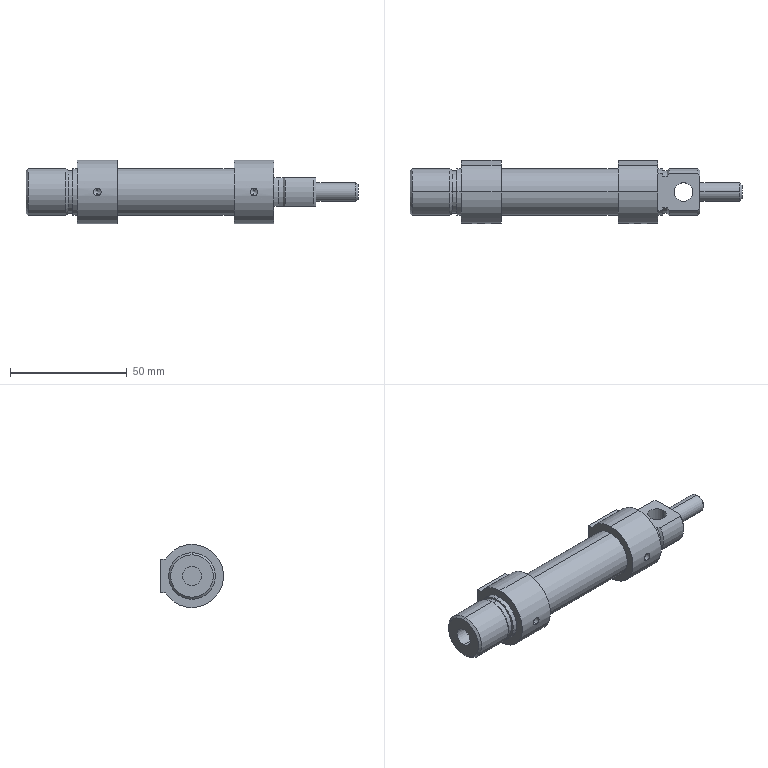Part | STEP file | 9123_DGS_16_10_P_z_HI | 2 solids | 77 faces | box 142 x 27 x 27 mm | volume 38230 mm3 | cylinder 36 | plane 23 | cone 18 | commonest cylinder face diameters 20 x10 8 x6 27 x6 3.3 x4 8.566 x4 18.159 x4